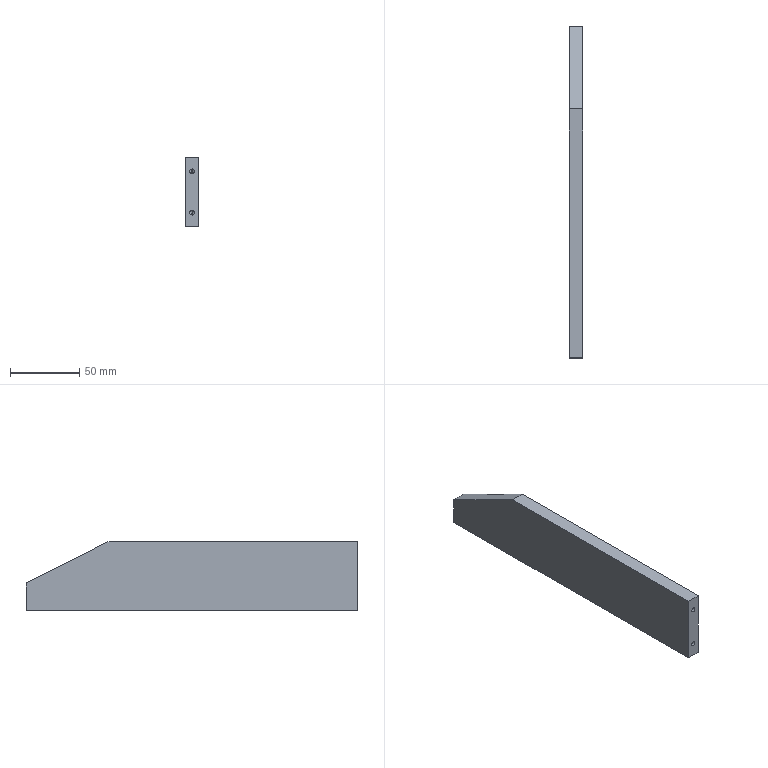Part | SolidWorks | features HoleWzd 2, Chamfer 1, Extrusion 1 | 1 solid | 31 faces | box 10 x 240 x 50 mm | volume 110213 mm3 | cylinder 12 | cone 12 | plane 7 | commonest cylinder face diameters 3.3 x12
STEP:
#1=CARTESIAN_POINT('',(0.,-105.,11.65));
#2=VERTEX_POINT('',#1);
#3=CARTESIAN_POINT('',(0.,-105.,8.35));
#4=VERTEX_POINT('',#3);
#5=CARTESIAN_POINT('',(0.,-105.,10.));
#6=DIRECTION('',(0.,-1.,0.));
#7=DIRECTION('',(0.,0.,-1.));
#8=AXIS2_PLACEMENT_3D('',#5,#6,#7);
#9=CIRCLE('',#8,1.65);
#10=EDGE_CURVE('',#2,#4,#9,.T.);
#11=ORIENTED_EDGE('',*,*,#10,.F.);
#12=CARTESIAN_POINT('',(0.,-120.,11.65));
#13=VERTEX_POINT('',#12);
#14=CARTESIAN_POINT('',(0.,-120.,11.65));
#15=DIRECTION('',(0.,-1.,0.));
#16=VECTOR('',#15,1000.);
#17=LINE('',#14,#16);
#18=EDGE_CURVE('',#2,#13,#17,.T.);
#19=ORIENTED_EDGE('',*,*,#18,.T.);
#20=CARTESIAN_POINT('',(0.,-120.,8.35));
#21=VERTEX_POINT('',#20);
#22=CARTESIAN_POINT('',(0.,-120.,10.));
#23=DIRECTION('',(0.,-1.,0.));
#24=DIRECTION('',(0.,0.,-1.));
#25=AXIS2_PLACEMENT_3D('',#22,#23,#24);
#26=CIRCLE('',#25,1.65);
#27=EDGE_CURVE('',#13,#21,#26,.T.);
#28=ORIENTED_EDGE('',*,*,#27,.T.);
#29=CARTESIAN_POINT('',(0.,-120.,8.35));
#30=DIRECTION('',(0.,-1.,0.));
#31=VECTOR('',#30,1000.);
#32=LINE('',#29,#31);
#33=EDGE_CURVE('',#4,#21,#32,.T.);
#34=ORIENTED_EDGE('',*,*,#33,.F.);
#35=EDGE_LOOP('',(#11,#19,#28,#34));
#36=FACE_OUTER_BOUND('',#35,.T.);
#37=CARTESIAN_POINT('',(0.,-120.,10.));
#38=DIRECTION('',(0.,-1.,0.));
#39=DIRECTION('',(0.,0.,-1.));
#40=AXIS2_PLACEMENT_3D('',#37,#38,#39);
#41=CYLINDRICAL_SURFACE('',#40,1.65);
#42=ADVANCED_FACE('',(#36),#41,.F.);
#43=CARTESIAN_POINT('',(0.,-104.009,10.));
#44=VERTEX_POINT('',#43);
#45=CARTESIAN_POINT('',(0.,-105.,8.35));
#46=DIRECTION('',(0.,-0.515,-0.8572));
#47=VECTOR('',#46,1000.);
#48=LINE('',#45,#47);
#49=EDGE_CURVE('',#44,#4,#48,.T.);
#50=ORIENTED_EDGE('',*,*,#49,.F.);
#51=CARTESIAN_POINT('',(0.,-105.,11.65));
#52=DIRECTION('',(0.,-0.515,0.8572));
#53=VECTOR('',#52,1000.);
#54=LINE('',#51,#53);
#55=EDGE_CURVE('',#44,#2,#54,.T.);
#56=ORIENTED_EDGE('',*,*,#55,.T.);
#57=ORIENTED_EDGE('',*,*,#10,.T.);
#58=EDGE_LOOP('',(#50,#56,#57));
#59=FACE_OUTER_BOUND('',#58,.T.);
#60=CARTESIAN_POINT('',(0.,-105.,10.));
#61=DIRECTION('',(0.,-1.,0.));
#62=DIRECTION('',(0.,0.,-1.));
#63=AXIS2_PLACEMENT_3D('',#60,#61,#62);
#64=CONICAL_SURFACE('',#63,1.65,1.03);
#65=ADVANCED_FACE('',(#59),#64,.F.);
#66=CARTESIAN_POINT('',(0.,-105.,41.65));
#67=VERTEX_POINT('',#66);
#68=CARTESIAN_POINT('',(0.,-105.,38.35));
#69=VERTEX_POINT('',#68);
#70=CARTESIAN_POINT('',(0.,-105.,40.));
#71=DIRECTION('',(0.,-1.,0.));
#72=DIRECTION('',(0.,0.,-1.));
#73=AXIS2_PLACEMENT_3D('',#70,#71,#72);
#74=CIRCLE('',#73,1.65);
#75=EDGE_CURVE('',#67,#69,#74,.T.);
#76=ORIENTED_EDGE('',*,*,#75,.F.);
#77=CARTESIAN_POINT('',(0.,-120.,41.65));
#78=VERTEX_POINT('',#77);
#79=CARTESIAN_POINT('',(0.,-120.,41.65));
#80=DIRECTION('',(0.,-1.,0.));
#81=VECTOR('',#80,1000.);
#82=LINE('',#79,#81);
#83=EDGE_CURVE('',#67,#78,#82,.T.);
#84=ORIENTED_EDGE('',*,*,#83,.T.);
#85=CARTESIAN_POINT('',(0.,-120.,38.35));
#86=VERTEX_POINT('',#85);
#87=CARTESIAN_POINT('',(0.,-120.,40.));
#88=DIRECTION('',(0.,-1.,0.));
#89=DIRECTION('',(0.,0.,-1.));
#90=AXIS2_PLACEMENT_3D('',#87,#88,#89);
#91=CIRCLE('',#90,1.65);
#92=EDGE_CURVE('',#78,#86,#91,.T.);
#93=ORIENTED_EDGE('',*,*,#92,.T.);
#94=CARTESIAN_POINT('',(0.,-120.,38.35));
#95=DIRECTION('',(0.,-1.,0.));
#96=VECTOR('',#95,1000.);
#97=LINE('',#94,#96);
#98=EDGE_CURVE('',#69,#86,#97,.T.);
#99=ORIENTED_EDGE('',*,*,#98,.F.);
#100=EDGE_LOOP('',(#76,#84,#93,#99));
#101=FACE_OUTER_BOUND('',#100,.T.);
#102=CARTESIAN_POINT('',(0.,-120.,40.));
#103=DIRECTION('',(0.,-1.,0.));
#104=DIRECTION('',(0.,0.,-1.));
#105=AXIS2_PLACEMENT_3D('',#102,#103,#104);
#106=CYLINDRICAL_SURFACE('',#105,1.65);
#107=ADVANCED_FACE('',(#101),#106,.F.);
#108=CARTESIAN_POINT('',(0.,-104.009,40.));
#109=VERTEX_POINT('',#108);
#110=CARTESIAN_POINT('',(0.,-105.,38.35));
#111=DIRECTION('',(0.,-0.515,-0.8572));
#112=VECTOR('',#111,1000.);
#113=LINE('',#110,#112);
#114=EDGE_CURVE('',#109,#69,#113,.T.);
#115=ORIENTED_EDGE('',*,*,#114,.F.);
#116=CARTESIAN_POINT('',(0.,-105.,41.65));
#117=DIRECTION('',(0.,-0.515,0.8572));
#118=VECTOR('',#117,1000.);
#119=LINE('',#116,#118);
#120=EDGE_CURVE('',#109,#67,#119,.T.);
#121=ORIENTED_EDGE('',*,*,#120,.T.);
#122=ORIENTED_EDGE('',*,*,#75,.T.);
#123=EDGE_LOOP('',(#115,#121,#122));
#124=FACE_OUTER_BOUND('',#123,.T.);
#125=CARTESIAN_POINT('',(0.,-105.,40.));
#126=DIRECTION('',(0.,-1.,0.));
#127=DIRECTION('',(0.,0.,-1.));
#128=AXIS2_PLACEMENT_3D('',#125,#126,#127);
#129=CONICAL_SURFACE('',#128,1.65,1.03);
#130=ADVANCED_FACE('',(#124),#129,.F.);
#131=CARTESIAN_POINT('',(1.65,97.5,15.));
#132=VERTEX_POINT('',#131);
#133=CARTESIAN_POINT('',(-1.65,97.5,15.));
#134=VERTEX_POINT('',#133);
#135=CARTESIAN_POINT('',(0.,97.5,15.));
#136=DIRECTION('',(0.,0.,-1.));
#137=DIRECTION('',(-1.,0.,0.));
#138=AXIS2_PLACEMENT_3D('',#135,#136,#137);
#139=CIRCLE('',#138,1.65);
#140=EDGE_CURVE('',#132,#134,#139,.T.);
#141=ORIENTED_EDGE('',*,*,#140,.F.);
#142=CARTESIAN_POINT('',(1.65,97.5,0.));
#143=VERTEX_POINT('',#142);
#144=CARTESIAN_POINT('',(1.65,97.5,0.));
#145=DIRECTION('',(0.,0.,-1.));
#146=VECTOR('',#145,1000.);
#147=LINE('',#144,#146);
#148=EDGE_CURVE('',#132,#143,#147,.T.);
#149=ORIENTED_EDGE('',*,*,#148,.T.);
#150=CARTESIAN_POINT('',(-1.65,97.5,0.));
#151=VERTEX_POINT('',#150);
#152=CARTESIAN_POINT('',(0.,97.5,0.));
#153=DIRECTION('',(0.,0.,-1.));
#154=DIRECTION('',(-1.,0.,0.));
#155=AXIS2_PLACEMENT_3D('',#152,#153,#154);
#156=CIRCLE('',#155,1.65);
#157=EDGE_CURVE('',#143,#151,#156,.T.);
#158=ORIENTED_EDGE('',*,*,#157,.T.);
#159=CARTESIAN_POINT('',(-1.65,97.5,0.));
#160=DIRECTION('',(0.,0.,-1.));
#161=VECTOR('',#160,1000.);
#162=LINE('',#159,#161);
#163=EDGE_CURVE('',#134,#151,#162,.T.);
#164=ORIENTED_EDGE('',*,*,#163,.F.);
#165=EDGE_LOOP('',(#141,#149,#158,#164));
#166=FACE_OUTER_BOUND('',#165,.T.);
#167=CARTESIAN_POINT('',(0.,97.5,0.));
#168=DIRECTION('',(0.,0.,-1.));
#169=DIRECTION('',(-1.,0.,0.));
#170=AXIS2_PLACEMENT_3D('',#167,#168,#169);
#171=CYLINDRICAL_SURFACE('',#170,1.65);
#172=ADVANCED_FACE('',(#166),#171,.F.);
#173=CARTESIAN_POINT('',(0.,97.5,15.991));
#174=VERTEX_POINT('',#173);
#175=CARTESIAN_POINT('',(-1.65,97.5,15.));
#176=DIRECTION('',(-0.8572,0.,-0.515));
#177=VECTOR('',#176,1000.);
#178=LINE('',#175,#177);
#179=EDGE_CURVE('',#174,#134,#178,.T.);
#180=ORIENTED_EDGE('',*,*,#179,.F.);
#181=CARTESIAN_POINT('',(1.65,97.5,15.));
#182=DIRECTION('',(0.8572,0.,-0.515));
#183=VECTOR('',#182,1000.);
#184=LINE('',#181,#183);
#185=EDGE_CURVE('',#174,#132,#184,.T.);
#186=ORIENTED_EDGE('',*,*,#185,.T.);
#187=ORIENTED_EDGE('',*,*,#140,.T.);
#188=EDGE_LOOP('',(#180,#186,#187));
#189=FACE_OUTER_BOUND('',#188,.T.);
#190=CARTESIAN_POINT('',(0.,97.5,15.));
#191=DIRECTION('',(0.,0.,-1.));
#192=DIRECTION('',(-1.,0.,0.));
#193=AXIS2_PLACEMENT_3D('',#190,#191,#192);
#194=CONICAL_SURFACE('',#193,1.65,1.03);
#195=ADVANCED_FACE('',(#189),#194,.F.);
#196=CARTESIAN_POINT('',(1.65,32.5,15.));
#197=VERTEX_POINT('',#196);
#198=CARTESIAN_POINT('',(-1.65,32.5,15.));
#199=VERTEX_POINT('',#198);
#200=CARTESIAN_POINT('',(0.,32.5,15.));
#201=DIRECTION('',(0.,0.,-1.));
#202=DIRECTION('',(-1.,0.,0.));
#203=AXIS2_PLACEMENT_3D('',#200,#201,#202);
#204=CIRCLE('',#203,1.65);
#205=EDGE_CURVE('',#197,#199,#204,.T.);
#206=ORIENTED_EDGE('',*,*,#205,.F.);
#207=CARTESIAN_POINT('',(1.65,32.5,0.));
#208=VERTEX_POINT('',#207);
#209=CARTESIAN_POINT('',(1.65,32.5,0.));
#210=DIRECTION('',(0.,0.,-1.));
#211=VECTOR('',#210,1000.);
#212=LINE('',#209,#211);
#213=EDGE_CURVE('',#197,#208,#212,.T.);
#214=ORIENTED_EDGE('',*,*,#213,.T.);
#215=CARTESIAN_POINT('',(-1.65,32.5,0.));
#216=VERTEX_POINT('',#215);
#217=CARTESIAN_POINT('',(0.,32.5,0.));
#218=DIRECTION('',(0.,0.,-1.));
#219=DIRECTION('',(-1.,0.,0.));
#220=AXIS2_PLACEMENT_3D('',#217,#218,#219);
#221=CIRCLE('',#220,1.65);
#222=EDGE_CURVE('',#208,#216,#221,.T.);
#223=ORIENTED_EDGE('',*,*,#222,.T.);
#224=CARTESIAN_POINT('',(-1.65,32.5,0.));
#225=DIRECTION('',(0.,0.,-1.));
#226=VECTOR('',#225,1000.);
#227=LINE('',#224,#226);
#228=EDGE_CURVE('',#199,#216,#227,.T.);
#229=ORIENTED_EDGE('',*,*,#228,.F.);
#230=EDGE_LOOP('',(#206,#214,#223,#229));
#231=FACE_OUTER_BOUND('',#230,.T.);
#232=CARTESIAN_POINT('',(0.,32.5,0.));
#233=DIRECTION('',(0.,0.,-1.));
#234=DIRECTION('',(-1.,0.,0.));
#235=AXIS2_PLACEMENT_3D('',#232,#233,#234);
#236=CYLINDRICAL_SURFACE('',#235,1.65);
#237=ADVANCED_FACE('',(#231),#236,.F.);
#238=CARTESIAN_POINT('',(0.,32.5,15.991));
#239=VERTEX_POINT('',#238);
#240=CARTESIAN_POINT('',(-1.65,32.5,15.));
#241=DIRECTION('',(-0.8572,0.,-0.515));
#242=VECTOR('',#241,1000.);
#243=LINE('',#240,#242);
#244=EDGE_CURVE('',#239,#199,#243,.T.);
#245=ORIENTED_EDGE('',*,*,#244,.F.);
#246=CARTESIAN_POINT('',(1.65,32.5,15.));
#247=DIRECTION('',(0.8572,0.,-0.515));
#248=VECTOR('',#247,1000.);
#249=LINE('',#246,#248);
#250=EDGE_CURVE('',#239,#197,#249,.T.);
#251=ORIENTED_EDGE('',*,*,#250,.T.);
#252=ORIENTED_EDGE('',*,*,#205,.T.);
#253=EDGE_LOOP('',(#245,#251,#252));
#254=FACE_OUTER_BOUND('',#253,.T.);
#255=CARTESIAN_POINT('',(0.,32.5,15.));
#256=DIRECTION('',(0.,0.,-1.));
#257=DIRECTION('',(-1.,0.,0.));
#258=AXIS2_PLACEMENT_3D('',#255,#256,#257);
#259=CONICAL_SURFACE('',#258,1.65,1.03);
#260=ADVANCED_FACE('',(#254),#259,.F.);
#261=CARTESIAN_POINT('',(1.65,-32.5,15.));
#262=VERTEX_POINT('',#261);
#263=CARTESIAN_POINT('',(-1.65,-32.5,15.));
#264=VERTEX_POINT('',#263);
#265=CARTESIAN_POINT('',(0.,-32.5,15.));
#266=DIRECTION('',(0.,0.,-1.));
#267=DIRECTION('',(-1.,0.,0.));
#268=AXIS2_PLACEMENT_3D('',#265,#266,#267);
#269=CIRCLE('',#268,1.65);
#270=EDGE_CURVE('',#262,#264,#269,.T.);
#271=ORIENTED_EDGE('',*,*,#270,.F.);
#272=CARTESIAN_POINT('',(1.65,-32.5,0.));
#273=VERTEX_POINT('',#272);
#274=CARTESIAN_POINT('',(1.65,-32.5,0.));
#275=DIRECTION('',(0.,0.,-1.));
#276=VECTOR('',#275,1000.);
#277=LINE('',#274,#276);
#278=EDGE_CURVE('',#262,#273,#277,.T.);
#279=ORIENTED_EDGE('',*,*,#278,.T.);
#280=CARTESIAN_POINT('',(-1.65,-32.5,0.));
#281=VERTEX_POINT('',#280);
#282=CARTESIAN_POINT('',(0.,-32.5,0.));
#283=DIRECTION('',(0.,0.,-1.));
#284=DIRECTION('',(-1.,0.,0.));
#285=AXIS2_PLACEMENT_3D('',#282,#283,#284);
#286=CIRCLE('',#285,1.65);
#287=EDGE_CURVE('',#273,#281,#286,.T.);
#288=ORIENTED_EDGE('',*,*,#287,.T.);
#289=CARTESIAN_POINT('',(-1.65,-32.5,0.));
#290=DIRECTION('',(0.,0.,-1.));
#291=VECTOR('',#290,1000.);
#292=LINE('',#289,#291);
#293=EDGE_CURVE('',#264,#281,#292,.T.);
#294=ORIENTED_EDGE('',*,*,#293,.F.);
#295=EDGE_LOOP('',(#271,#279,#288,#294));
#296=FACE_OUTER_BOUND('',#295,.T.);
#297=CARTESIAN_POINT('',(0.,-32.5,0.));
#298=DIRECTION('',(0.,0.,-1.));
#299=DIRECTION('',(-1.,0.,0.));
#300=AXIS2_PLACEMENT_3D('',#297,#298,#299);
#301=CYLINDRICAL_SURFACE('',#300,1.65);
#302=ADVANCED_FACE('',(#296),#301,.F.);
#303=CARTESIAN_POINT('',(0.,-32.5,15.991));
#304=VERTEX_POINT('',#303);
#305=CARTESIAN_POINT('',(-1.65,-32.5,15.));
#306=DIRECTION('',(-0.8572,0.,-0.515));
#307=VECTOR('',#306,1000.);
#308=LINE('',#305,#307);
#309=EDGE_CURVE('',#304,#264,#308,.T.);
#310=ORIENTED_EDGE('',*,*,#309,.F.);
#311=CARTESIAN_POINT('',(1.65,-32.5,15.));
#312=DIRECTION('',(0.8572,0.,-0.515));
#313=VECTOR('',#312,1000.);
#314=LINE('',#311,#313);
#315=EDGE_CURVE('',#304,#262,#314,.T.);
#316=ORIENTED_EDGE('',*,*,#315,.T.);
#317=ORIENTED_EDGE('',*,*,#270,.T.);
#318=EDGE_LOOP('',(#310,#316,#317));
#319=FACE_OUTER_BOUND('',#318,.T.);
#320=CARTESIAN_POINT('',(0.,-32.5,15.));
#321=DIRECTION('',(0.,0.,-1.));
#322=DIRECTION('',(-1.,0.,0.));
#323=AXIS2_PLACEMENT_3D('',#320,#321,#322);
#324=CONICAL_SURFACE('',#323,1.65,1.03);
#325=ADVANCED_FACE('',(#319),#324,.F.);
#326=CARTESIAN_POINT('',(1.65,-97.5,15.));
#327=VERTEX_POINT('',#326);
#328=CARTESIAN_POINT('',(-1.65,-97.5,15.));
#329=VERTEX_POINT('',#328);
#330=CARTESIAN_POINT('',(0.,-97.5,15.));
#331=DIRECTION('',(0.,0.,-1.));
#332=DIRECTION('',(-1.,0.,0.));
#333=AXIS2_PLACEMENT_3D('',#330,#331,#332);
#334=CIRCLE('',#333,1.65);
#335=EDGE_CURVE('',#327,#329,#334,.T.);
#336=ORIENTED_EDGE('',*,*,#335,.F.);
#337=CARTESIAN_POINT('',(1.65,-97.5,0.));
#338=VERTEX_POINT('',#337);
#339=CARTESIAN_POINT('',(1.65,-97.5,0.));
#340=DIRECTION('',(0.,0.,-1.));
#341=VECTOR('',#340,1000.);
#342=LINE('',#339,#341);
#343=EDGE_CURVE('',#327,#338,#342,.T.);
#344=ORIENTED_EDGE('',*,*,#343,.T.);
#345=CARTESIAN_POINT('',(-1.65,-97.5,0.));
#346=VERTEX_POINT('',#345);
#347=CARTESIAN_POINT('',(0.,-97.5,0.));
#348=DIRECTION('',(0.,0.,-1.));
#349=DIRECTION('',(-1.,0.,0.));
#350=AXIS2_PLACEMENT_3D('',#347,#348,#349);
#351=CIRCLE('',#350,1.65);
#352=EDGE_CURVE('',#338,#346,#351,.T.);
#353=ORIENTED_EDGE('',*,*,#352,.T.);
#354=CARTESIAN_POINT('',(-1.65,-97.5,0.));
#355=DIRECTION('',(0.,0.,-1.));
#356=VECTOR('',#355,1000.);
#357=LINE('',#354,#356);
#358=EDGE_CURVE('',#329,#346,#357,.T.);
#359=ORIENTED_EDGE('',*,*,#358,.F.);
#360=EDGE_LOOP('',(#336,#344,#353,#359));
#361=FACE_OUTER_BOUND('',#360,.T.);
#362=CARTESIAN_POINT('',(0.,-97.5,0.));
#363=DIRECTION('',(0.,0.,-1.));
#364=DIRECTION('',(-1.,0.,0.));
#365=AXIS2_PLACEMENT_3D('',#362,#363,#364);
#366=CYLINDRICAL_SURFACE('',#365,1.65);
#367=ADVANCED_FACE('',(#361),#366,.F.);
#368=CARTESIAN_POINT('',(0.,-97.5,15.991));
#369=VERTEX_POINT('',#368);
#370=CARTESIAN_POINT('',(-1.65,-97.5,15.));
#371=DIRECTION('',(-0.8572,0.,-0.515));
#372=VECTOR('',#371,1000.);
#373=LINE('',#370,#372);
#374=EDGE_CURVE('',#369,#329,#373,.T.);
#375=ORIENTED_EDGE('',*,*,#374,.F.);
#376=CARTESIAN_POINT('',(1.65,-97.5,15.));
#377=DIRECTION('',(0.8572,0.,-0.515));
#378=VECTOR('',#377,1000.);
#379=LINE('',#376,#378);
#380=EDGE_CURVE('',#369,#327,#379,.T.);
#381=ORIENTED_EDGE('',*,*,#380,.T.);
#382=ORIENTED_EDGE('',*,*,#335,.T.);
#383=EDGE_LOOP('',(#375,#381,#382));
#384=FACE_OUTER_BOUND('',#383,.T.);
#385=CARTESIAN_POINT('',(0.,-97.5,15.));
#386=DIRECTION('',(0.,0.,-1.));
#387=DIRECTION('',(-1.,0.,0.));
#388=AXIS2_PLACEMENT_3D('',#385,#386,#387);
#389=CONICAL_SURFACE('',#388,1.65,1.03);
#390=ADVANCED_FACE('',(#384),#389,.F.);
#391=CARTESIAN_POINT('',(5.,120.,20.));
#392=VERTEX_POINT('',#391);
#393=CARTESIAN_POINT('',(5.,120.,0.));
#394=VERTEX_POINT('',#393);
#395=CARTESIAN_POINT('',(5.,120.,50.));
#396=DIRECTION('',(0.,0.,-1.));
#397=VECTOR('',#396,1000.);
#398=LINE('',#395,#397);
#399=EDGE_CURVE('',#392,#394,#398,.T.);
#400=ORIENTED_EDGE('',*,*,#399,.F.);
#401=CARTESIAN_POINT('',(5.,60.,50.));
#402=VERTEX_POINT('',#401);
#403=CARTESIAN_POINT('',(5.,60.,50.));
#404=DIRECTION('',(0.,-0.8944,0.4472));
#405=VECTOR('',#404,1000.);
#406=LINE('',#403,#405);
#407=EDGE_CURVE('',#392,#402,#406,.T.);
#408=ORIENTED_EDGE('',*,*,#407,.T.);
#409=CARTESIAN_POINT('',(5.,-120.,50.));
#410=VERTEX_POINT('',#409);
#411=CARTESIAN_POINT('',(5.,120.,50.));
#412=DIRECTION('',(0.,1.,0.));
#413=VECTOR('',#412,1000.);
#414=LINE('',#411,#413);
#415=EDGE_CURVE('',#410,#402,#414,.T.);
#416=ORIENTED_EDGE('',*,*,#415,.F.);
#417=CARTESIAN_POINT('',(5.,-120.,0.));
#418=VERTEX_POINT('',#417);
#419=CARTESIAN_POINT('',(5.,-120.,50.));
#420=DIRECTION('',(0.,0.,-1.));
#421=VECTOR('',#420,1000.);
#422=LINE('',#419,#421);
#423=EDGE_CURVE('',#410,#418,#422,.T.);
#424=ORIENTED_EDGE('',*,*,#423,.T.);
#425=CARTESIAN_POINT('',(5.,120.,0.));
#426=DIRECTION('',(0.,1.,0.));
#427=VECTOR('',#426,1000.);
#428=LINE('',#425,#427);
#429=EDGE_CURVE('',#418,#394,#428,.T.);
#430=ORIENTED_EDGE('',*,*,#429,.T.);
#431=EDGE_LOOP('',(#400,#408,#416,#424,#430));
#432=FACE_OUTER_BOUND('',#431,.T.);
#433=CARTESIAN_POINT('',(5.,120.,50.));
#434=DIRECTION('',(-1.,0.,0.));
#435=DIRECTION('',(0.,-1.,0.));
#436=AXIS2_PLACEMENT_3D('',#433,#434,#435);
#437=PLANE('',#436);
#438=ADVANCED_FACE('',(#432),#437,.F.);
#439=CARTESIAN_POINT('',(-5.,120.,20.));
#440=VERTEX_POINT('',#439);
#441=CARTESIAN_POINT('',(-5.,120.,0.));
#442=VERTEX_POINT('',#441);
#443=CARTESIAN_POINT('',(-5.,120.,50.));
#444=DIRECTION('',(0.,0.,-1.));
#445=VECTOR('',#444,1000.);
#446=LINE('',#443,#445);
#447=EDGE_CURVE('',#440,#442,#446,.T.);
#448=ORIENTED_EDGE('',*,*,#447,.F.);
#449=CARTESIAN_POINT('',(5.,120.,20.));
#450=DIRECTION('',(1.,0.,0.));
#451=VECTOR('',#450,1000.);
#452=LINE('',#449,#451);
#453=EDGE_CURVE('',#440,#392,#452,.T.);
#454=ORIENTED_EDGE('',*,*,#453,.T.);
#455=ORIENTED_EDGE('',*,*,#399,.T.);
#456=CARTESIAN_POINT('',(-5.,120.,0.));
#457=DIRECTION('',(-1.,0.,0.));
#458=VECTOR('',#457,1000.);
#459=LINE('',#456,#458);
#460=EDGE_CURVE('',#394,#442,#459,.T.);
#461=ORIENTED_EDGE('',*,*,#460,.T.);
#462=EDGE_LOOP('',(#448,#454,#455,#461));
#463=FACE_OUTER_BOUND('',#462,.T.);
#464=CARTESIAN_POINT('',(-5.,120.,50.));
#465=DIRECTION('',(0.,-1.,0.));
#466=DIRECTION('',(0.,0.,-1.));
#467=AXIS2_PLACEMENT_3D('',#464,#465,#466);
#468=PLANE('',#467);
#469=ADVANCED_FACE('',(#463),#468,.F.);
#470=CARTESIAN_POINT('',(-5.,60.,50.));
#471=VERTEX_POINT('',#470);
#472=CARTESIAN_POINT('',(-5.,-120.,50.));
#473=VERTEX_POINT('',#472);
#474=CARTESIAN_POINT('',(-5.,120.,50.));
#475=DIRECTION('',(0.,-1.,0.));
#476=VECTOR('',#475,1000.);
#477=LINE('',#474,#476);
#478=EDGE_CURVE('',#471,#473,#477,.T.);
#479=ORIENTED_EDGE('',*,*,#478,.F.);
#480=CARTESIAN_POINT('',(-5.,60.,50.));
#481=DIRECTION('',(0.,0.8944,-0.4472));
#482=VECTOR('',#481,1000.);
#483=LINE('',#480,#482);
#484=EDGE_CURVE('',#471,#440,#483,.T.);
#485=ORIENTED_EDGE('',*,*,#484,.T.);
#486=ORIENTED_EDGE('',*,*,#447,.T.);
#487=CARTESIAN_POINT('',(-5.,-120.,0.));
#488=VERTEX_POINT('',#487);
#489=CARTESIAN_POINT('',(-5.,120.,0.));
#490=DIRECTION('',(0.,-1.,0.));
#491=VECTOR('',#490,1000.);
#492=LINE('',#489,#491);
#493=EDGE_CURVE('',#442,#488,#492,.T.);
#494=ORIENTED_EDGE('',*,*,#493,.T.);
#495=CARTESIAN_POINT('',(-5.,-120.,50.));
#496=DIRECTION('',(0.,0.,-1.));
#497=VECTOR('',#496,1000.);
#498=LINE('',#495,#497);
#499=EDGE_CURVE('',#473,#488,#498,.T.);
#500=ORIENTED_EDGE('',*,*,#499,.F.);
#501=EDGE_LOOP('',(#479,#485,#486,#494,#500));
#502=FACE_OUTER_BOUND('',#501,.T.);
#503=CARTESIAN_POINT('',(-5.,120.,50.));
#504=DIRECTION('',(1.,0.,0.));
#505=DIRECTION('',(0.,1.,0.));
#506=AXIS2_PLACEMENT_3D('',#503,#504,#505);
#507=PLANE('',#506);
#508=ADVANCED_FACE('',(#502),#507,.F.);
#509=CARTESIAN_POINT('',(0.,-120.,10.));
#510=DIRECTION('',(0.,-1.,0.));
#511=DIRECTION('',(0.,0.,-1.));
#512=AXIS2_PLACEMENT_3D('',#509,#510,#511);
#513=CIRCLE('',#512,1.65);
#514=EDGE_CURVE('',#21,#13,#513,.T.);
#515=ORIENTED_EDGE('',*,*,#514,.F.);
#516=ORIENTED_EDGE('',*,*,#27,.F.);
#517=EDGE_LOOP('',(#515,#516));
#518=FACE_BOUND('',#517,.T.);
#519=CARTESIAN_POINT('',(0.,-120.,40.));
#520=DIRECTION('',(0.,-1.,0.));
#521=DIRECTION('',(0.,0.,-1.));
#522=AXIS2_PLACEMENT_3D('',#519,#520,#521);
#523=CIRCLE('',#522,1.65);
#524=EDGE_CURVE('',#86,#78,#523,.T.);
#525=ORIENTED_EDGE('',*,*,#524,.F.);
#526=ORIENTED_EDGE('',*,*,#92,.F.);
#527=EDGE_LOOP('',(#525,#526));
#528=FACE_BOUND('',#527,.T.);
#529=CARTESIAN_POINT('',(-5.,-120.,0.));
#530=DIRECTION('',(1.,0.,0.));
#531=VECTOR('',#530,1000.);
#532=LINE('',#529,#531);
#533=EDGE_CURVE('',#488,#418,#532,.T.);
#534=ORIENTED_EDGE('',*,*,#533,.T.);
#535=ORIENTED_EDGE('',*,*,#423,.F.);
#536=CARTESIAN_POINT('',(-5.,-120.,50.));
#537=DIRECTION('',(1.,0.,0.));
#538=VECTOR('',#537,1000.);
#539=LINE('',#536,#538);
#540=EDGE_CURVE('',#473,#410,#539,.T.);
#541=ORIENTED_EDGE('',*,*,#540,.F.);
#542=ORIENTED_EDGE('',*,*,#499,.T.);
#543=EDGE_LOOP('',(#534,#535,#541,#542));
#544=FACE_OUTER_BOUND('',#543,.T.);
#545=CARTESIAN_POINT('',(-5.,-120.,50.));
#546=DIRECTION('',(0.,1.,0.));
#547=DIRECTION('',(0.,0.,1.));
#548=AXIS2_PLACEMENT_3D('',#545,#546,#547);
#549=PLANE('',#548);
#550=ADVANCED_FACE('',(#518,#528,#544),#549,.F.);
#551=ORIENTED_EDGE('',*,*,#415,.T.);
#552=CARTESIAN_POINT('',(-5.,60.,50.));
#553=DIRECTION('',(-1.,0.,0.));
#554=VECTOR('',#553,1000.);
#555=LINE('',#552,#554);
#556=EDGE_CURVE('',#402,#471,#555,.T.);
#557=ORIENTED_EDGE('',*,*,#556,.T.);
#558=ORIENTED_EDGE('',*,*,#478,.T.);
#559=ORIENTED_EDGE('',*,*,#540,.T.);
#560=EDGE_LOOP('',(#551,#557,#558,#559));
#561=FACE_OUTER_BOUND('',#560,.T.);
#562=CARTESIAN_POINT('',(0.,0.,50.));
#563=DIRECTION('',(0.,0.,1.));
#564=DIRECTION('',(1.,0.,0.));
#565=AXIS2_PLACEMENT_3D('',#562,#563,#564);
#566=PLANE('',#565);
#567=ADVANCED_FACE('',(#561),#566,.T.);
#568=CARTESIAN_POINT('',(0.,97.5,0.));
#569=DIRECTION('',(0.,0.,-1.));
#570=DIRECTION('',(-1.,0.,0.));
#571=AXIS2_PLACEMENT_3D('',#568,#569,#570);
#572=CIRCLE('',#571,1.65);
#573=EDGE_CURVE('',#151,#143,#572,.T.);
#574=ORIENTED_EDGE('',*,*,#573,.F.);
#575=ORIENTED_EDGE('',*,*,#157,.F.);
#576=EDGE_LOOP('',(#574,#575));
#577=FACE_BOUND('',#576,.T.);
#578=CARTESIAN_POINT('',(0.,32.5,0.));
#579=DIRECTION('',(0.,0.,-1.));
#580=DIRECTION('',(-1.,0.,0.));
#581=AXIS2_PLACEMENT_3D('',#578,#579,#580);
#582=CIRCLE('',#581,1.65);
#583=EDGE_CURVE('',#216,#208,#582,.T.);
#584=ORIENTED_EDGE('',*,*,#583,.F.);
#585=ORIENTED_EDGE('',*,*,#222,.F.);
#586=EDGE_LOOP('',(#584,#585));
#587=FACE_BOUND('',#586,.T.);
#588=CARTESIAN_POINT('',(0.,-32.5,0.));
#589=DIRECTION('',(0.,0.,-1.));
#590=DIRECTION('',(-1.,0.,0.));
#591=AXIS2_PLACEMENT_3D('',#588,#589,#590);
#592=CIRCLE('',#591,1.65);
#593=EDGE_CURVE('',#281,#273,#592,.T.);
#594=ORIENTED_EDGE('',*,*,#593,.F.);
#595=ORIENTED_EDGE('',*,*,#287,.F.);
#596=EDGE_LOOP('',(#594,#595));
#597=FACE_BOUND('',#596,.T.);
#598=CARTESIAN_POINT('',(0.,-97.5,0.));
#599=DIRECTION('',(0.,0.,-1.));
#600=DIRECTION('',(-1.,0.,0.));
#601=AXIS2_PLACEMENT_3D('',#598,#599,#600);
#602=CIRCLE('',#601,1.65);
#603=EDGE_CURVE('',#346,#338,#602,.T.);
#604=ORIENTED_EDGE('',*,*,#603,.F.);
#605=ORIENTED_EDGE('',*,*,#352,.F.);
#606=EDGE_LOOP('',(#604,#605));
#607=FACE_BOUND('',#606,.T.);
#608=ORIENTED_EDGE('',*,*,#429,.F.);
#609=ORIENTED_EDGE('',*,*,#533,.F.);
#610=ORIENTED_EDGE('',*,*,#493,.F.);
#611=ORIENTED_EDGE('',*,*,#460,.F.);
#612=EDGE_LOOP('',(#608,#609,#610,#611));
#613=FACE_OUTER_BOUND('',#612,.T.);
#614=CARTESIAN_POINT('',(0.,0.,0.));
#615=DIRECTION('',(0.,0.,1.));
#616=DIRECTION('',(1.,0.,0.));
#617=AXIS2_PLACEMENT_3D('',#614,#615,#616);
#618=PLANE('',#617);
#619=ADVANCED_FACE('',(#577,#587,#597,#607,#613),#618,.F.);
#620=ORIENTED_EDGE('',*,*,#380,.F.);
#621=ORIENTED_EDGE('',*,*,#374,.T.);
#622=CARTESIAN_POINT('',(0.,-97.5,15.));
#623=DIRECTION('',(0.,0.,-1.));
#624=DIRECTION('',(-1.,0.,0.));
#625=AXIS2_PLACEMENT_3D('',#622,#623,#624);
#626=CIRCLE('',#625,1.65);
#627=EDGE_CURVE('',#329,#327,#626,.T.);
#628=ORIENTED_EDGE('',*,*,#627,.T.);
#629=EDGE_LOOP('',(#620,#621,#628));
#630=FACE_OUTER_BOUND('',#629,.T.);
#631=CARTESIAN_POINT('',(0.,-97.5,15.));
#632=DIRECTION('',(0.,0.,-1.));
#633=DIRECTION('',(-1.,0.,0.));
#634=AXIS2_PLACEMENT_3D('',#631,#632,#633);
#635=CONICAL_SURFACE('',#634,1.65,1.03);
#636=ADVANCED_FACE('',(#630),#635,.F.);
#637=ORIENTED_EDGE('',*,*,#343,.F.);
#638=ORIENTED_EDGE('',*,*,#627,.F.);
#639=ORIENTED_EDGE('',*,*,#358,.T.);
#640=ORIENTED_EDGE('',*,*,#603,.T.);
#641=EDGE_LOOP('',(#637,#638,#639,#640));
#642=FACE_OUTER_BOUND('',#641,.T.);
#643=CARTESIAN_POINT('',(0.,-97.5,0.));
#644=DIRECTION('',(0.,0.,-1.));
#645=DIRECTION('',(-1.,0.,0.));
#646=AXIS2_PLACEMENT_3D('',#643,#644,#645);
#647=CYLINDRICAL_SURFACE('',#646,1.65);
#648=ADVANCED_FACE('',(#642),#647,.F.);
#649=ORIENTED_EDGE('',*,*,#315,.F.);
#650=ORIENTED_EDGE('',*,*,#309,.T.);
#651=CARTESIAN_POINT('',(0.,-32.5,15.));
#652=DIRECTION('',(0.,0.,-1.));
#653=DIRECTION('',(-1.,0.,0.));
#654=AXIS2_PLACEMENT_3D('',#651,#652,#653);
#655=CIRCLE('',#654,1.65);
#656=EDGE_CURVE('',#264,#262,#655,.T.);
#657=ORIENTED_EDGE('',*,*,#656,.T.);
#658=EDGE_LOOP('',(#649,#650,#657));
#659=FACE_OUTER_BOUND('',#658,.T.);
#660=CARTESIAN_POINT('',(0.,-32.5,15.));
#661=DIRECTION('',(0.,0.,-1.));
#662=DIRECTION('',(-1.,0.,0.));
#663=AXIS2_PLACEMENT_3D('',#660,#661,#662);
#664=CONICAL_SURFACE('',#663,1.65,1.03);
#665=ADVANCED_FACE('',(#659),#664,.F.);
#666=ORIENTED_EDGE('',*,*,#278,.F.);
#667=ORIENTED_EDGE('',*,*,#656,.F.);
#668=ORIENTED_EDGE('',*,*,#293,.T.);
#669=ORIENTED_EDGE('',*,*,#593,.T.);
#670=EDGE_LOOP('',(#666,#667,#668,#669));
#671=FACE_OUTER_BOUND('',#670,.T.);
#672=CARTESIAN_POINT('',(0.,-32.5,0.));
#673=DIRECTION('',(0.,0.,-1.));
#674=DIRECTION('',(-1.,0.,0.));
#675=AXIS2_PLACEMENT_3D('',#672,#673,#674);
#676=CYLINDRICAL_SURFACE('',#675,1.65);
#677=ADVANCED_FACE('',(#671),#676,.F.);
#678=ORIENTED_EDGE('',*,*,#250,.F.);
#679=ORIENTED_EDGE('',*,*,#244,.T.);
#680=CARTESIAN_POINT('',(0.,32.5,15.));
#681=DIRECTION('',(0.,0.,-1.));
#682=DIRECTION('',(-1.,0.,0.));
#683=AXIS2_PLACEMENT_3D('',#680,#681,#682);
#684=CIRCLE('',#683,1.65);
#685=EDGE_CURVE('',#199,#197,#684,.T.);
#686=ORIENTED_EDGE('',*,*,#685,.T.);
#687=EDGE_LOOP('',(#678,#679,#686));
#688=FACE_OUTER_BOUND('',#687,.T.);
#689=CARTESIAN_POINT('',(0.,32.5,15.));
#690=DIRECTION('',(0.,0.,-1.));
#691=DIRECTION('',(-1.,0.,0.));
#692=AXIS2_PLACEMENT_3D('',#689,#690,#691);
#693=CONICAL_SURFACE('',#692,1.65,1.03);
#694=ADVANCED_FACE('',(#688),#693,.F.);
#695=ORIENTED_EDGE('',*,*,#213,.F.);
#696=ORIENTED_EDGE('',*,*,#685,.F.);
#697=ORIENTED_EDGE('',*,*,#228,.T.);
#698=ORIENTED_EDGE('',*,*,#583,.T.);
#699=EDGE_LOOP('',(#695,#696,#697,#698));
#700=FACE_OUTER_BOUND('',#699,.T.);
#701=CARTESIAN_POINT('',(0.,32.5,0.));
#702=DIRECTION('',(0.,0.,-1.));
#703=DIRECTION('',(-1.,0.,0.));
#704=AXIS2_PLACEMENT_3D('',#701,#702,#703);
#705=CYLINDRICAL_SURFACE('',#704,1.65);
#706=ADVANCED_FACE('',(#700),#705,.F.);
#707=ORIENTED_EDGE('',*,*,#185,.F.);
#708=ORIENTED_EDGE('',*,*,#179,.T.);
#709=CARTESIAN_POINT('',(0.,97.5,15.));
#710=DIRECTION('',(0.,0.,-1.));
#711=DIRECTION('',(-1.,0.,0.));
#712=AXIS2_PLACEMENT_3D('',#709,#710,#711);
#713=CIRCLE('',#712,1.65);
#714=EDGE_CURVE('',#134,#132,#713,.T.);
#715=ORIENTED_EDGE('',*,*,#714,.T.);
#716=EDGE_LOOP('',(#707,#708,#715));
#717=FACE_OUTER_BOUND('',#716,.T.);
#718=CARTESIAN_POINT('',(0.,97.5,15.));
#719=DIRECTION('',(0.,0.,-1.));
#720=DIRECTION('',(-1.,0.,0.));
#721=AXIS2_PLACEMENT_3D('',#718,#719,#720);
#722=CONICAL_SURFACE('',#721,1.65,1.03);
#723=ADVANCED_FACE('',(#717),#722,.F.);
#724=ORIENTED_EDGE('',*,*,#148,.F.);
#725=ORIENTED_EDGE('',*,*,#714,.F.);
#726=ORIENTED_EDGE('',*,*,#163,.T.);
#727=ORIENTED_EDGE('',*,*,#573,.T.);
#728=EDGE_LOOP('',(#724,#725,#726,#727));
#729=FACE_OUTER_BOUND('',#728,.T.);
#730=CARTESIAN_POINT('',(0.,97.5,0.));
#731=DIRECTION('',(0.,0.,-1.));
#732=DIRECTION('',(-1.,0.,0.));
#733=AXIS2_PLACEMENT_3D('',#730,#731,#732);
#734=CYLINDRICAL_SURFACE('',#733,1.65);
#735=ADVANCED_FACE('',(#729),#734,.F.);
#736=ORIENTED_EDGE('',*,*,#120,.F.);
#737=ORIENTED_EDGE('',*,*,#114,.T.);
#738=CARTESIAN_POINT('',(0.,-105.,40.));
#739=DIRECTION('',(0.,-1.,0.));
#740=DIRECTION('',(0.,0.,-1.));
#741=AXIS2_PLACEMENT_3D('',#738,#739,#740);
#742=CIRCLE('',#741,1.65);
#743=EDGE_CURVE('',#69,#67,#742,.T.);
#744=ORIENTED_EDGE('',*,*,#743,.T.);
#745=EDGE_LOOP('',(#736,#737,#744));
#746=FACE_OUTER_BOUND('',#745,.T.);
#747=CARTESIAN_POINT('',(0.,-105.,40.));
#748=DIRECTION('',(0.,-1.,0.));
#749=DIRECTION('',(0.,0.,-1.));
#750=AXIS2_PLACEMENT_3D('',#747,#748,#749);
#751=CONICAL_SURFACE('',#750,1.65,1.03);
#752=ADVANCED_FACE('',(#746),#751,.F.);
#753=ORIENTED_EDGE('',*,*,#83,.F.);
#754=ORIENTED_EDGE('',*,*,#743,.F.);
#755=ORIENTED_EDGE('',*,*,#98,.T.);
#756=ORIENTED_EDGE('',*,*,#524,.T.);
#757=EDGE_LOOP('',(#753,#754,#755,#756));
#758=FACE_OUTER_BOUND('',#757,.T.);
#759=CARTESIAN_POINT('',(0.,-120.,40.));
#760=DIRECTION('',(0.,-1.,0.));
#761=DIRECTION('',(0.,0.,-1.));
#762=AXIS2_PLACEMENT_3D('',#759,#760,#761);
#763=CYLINDRICAL_SURFACE('',#762,1.65);
#764=ADVANCED_FACE('',(#758),#763,.F.);
#765=ORIENTED_EDGE('',*,*,#55,.F.);
#766=ORIENTED_EDGE('',*,*,#49,.T.);
#767=CARTESIAN_POINT('',(0.,-105.,10.));
#768=DIRECTION('',(0.,-1.,0.));
#769=DIRECTION('',(0.,0.,-1.));
#770=AXIS2_PLACEMENT_3D('',#767,#768,#769);
#771=CIRCLE('',#770,1.65);
#772=EDGE_CURVE('',#4,#2,#771,.T.);
#773=ORIENTED_EDGE('',*,*,#772,.T.);
#774=EDGE_LOOP('',(#765,#766,#773));
#775=FACE_OUTER_BOUND('',#774,.T.);
#776=CARTESIAN_POINT('',(0.,-105.,10.));
#777=DIRECTION('',(0.,-1.,0.));
#778=DIRECTION('',(0.,0.,-1.));
#779=AXIS2_PLACEMENT_3D('',#776,#777,#778);
#780=CONICAL_SURFACE('',#779,1.65,1.03);
#781=ADVANCED_FACE('',(#775),#780,.F.);
#782=ORIENTED_EDGE('',*,*,#18,.F.);
#783=ORIENTED_EDGE('',*,*,#772,.F.);
#784=ORIENTED_EDGE('',*,*,#33,.T.);
#785=ORIENTED_EDGE('',*,*,#514,.T.);
#786=EDGE_LOOP('',(#782,#783,#784,#785));
#787=FACE_OUTER_BOUND('',#786,.T.);
#788=CARTESIAN_POINT('',(0.,-120.,10.));
#789=DIRECTION('',(0.,-1.,0.));
#790=DIRECTION('',(0.,0.,-1.));
#791=AXIS2_PLACEMENT_3D('',#788,#789,#790);
#792=CYLINDRICAL_SURFACE('',#791,1.65);
#793=ADVANCED_FACE('',(#787),#792,.F.);
#794=ORIENTED_EDGE('',*,*,#407,.F.);
#795=ORIENTED_EDGE('',*,*,#453,.F.);
#796=ORIENTED_EDGE('',*,*,#484,.F.);
#797=ORIENTED_EDGE('',*,*,#556,.F.);
#798=EDGE_LOOP('',(#794,#795,#796,#797));
#799=FACE_OUTER_BOUND('',#798,.T.);
#800=CARTESIAN_POINT('',(0.,60.,50.));
#801=DIRECTION('',(0.,0.4472,0.8944));
#802=DIRECTION('',(1.,0.,0.));
#803=AXIS2_PLACEMENT_3D('',#800,#801,#802);
#804=PLANE('',#803);
#805=ADVANCED_FACE('',(#799),#804,.T.);
#806=CLOSED_SHELL('',(#42,#65,#107,#130,#172,#195,#237,#260,#302,#325,#367,#390,#438,#469,#508,#550,#567,#619,#636,#648,#665,#677,#694,#706,#723,#735,#752,#764,#781,#793,#805));
#807=MANIFOLD_SOLID_BREP('',#806);
#808=CARTESIAN_POINT('',(0.,0.,0.));
#809=DIRECTION('',(0.,0.,1.));
#810=DIRECTION('',(1.,0.,0.));
#811=AXIS2_PLACEMENT_3D('',#808,#809,#810);
#812=(LENGTH_UNIT()NAMED_UNIT(*)SI_UNIT(.MILLI.,.METRE.));
#813=UNCERTAINTY_MEASURE_WITH_UNIT(LENGTH_MEASURE(0.00001),#812,'','');
#814=(NAMED_UNIT(*)PLANE_ANGLE_UNIT()SI_UNIT($,.RADIAN.));
#815=(NAMED_UNIT(*)SI_UNIT($,.STERADIAN.)SOLID_ANGLE_UNIT());
#816=(GEOMETRIC_REPRESENTATION_CONTEXT(3)GLOBAL_UNCERTAINTY_ASSIGNED_CONTEXT((#813))GLOBAL_UNIT_ASSIGNED_CONTEXT((#812,#814,#815))REPRESENTATION_CONTEXT('',''));
#817=ADVANCED_BREP_SHAPE_REPRESENTATION('',(#807,#811),#816);